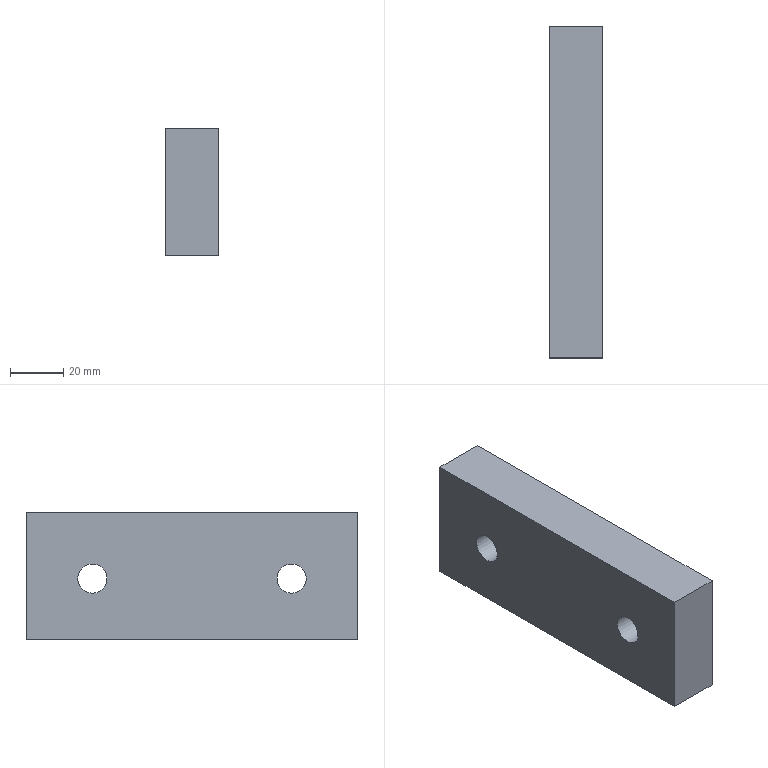Part | NX | features solid 2 | 1 solid | 12 faces | box 20 x 125 x 48 mm | volume 114744 mm3 | plane 8 | cylinder 4 | commonest cylinder face diameters 11 x2 17.5 x2
STEP:
#1=CARTESIAN_POINT('',(600.,560.,92.));
#2=VERTEX_POINT('',#1);
#3=CARTESIAN_POINT('',(580.,560.,92.));
#4=VERTEX_POINT('',#3);
#5=CARTESIAN_POINT('',(590.,560.,92.));
#6=DIRECTION('',(-1.,0.,0.));
#7=VECTOR('',#6,1000.);
#8=LINE('',#5,#7);
#9=EDGE_CURVE('',#2,#4,#8,.T.);
#10=ORIENTED_EDGE('',*,*,#9,.F.);
#11=CARTESIAN_POINT('',(600.,560.,140.));
#12=VERTEX_POINT('',#11);
#13=CARTESIAN_POINT('',(600.,560.,90.));
#14=DIRECTION('',(0.,0.,-1.));
#15=VECTOR('',#14,1000.);
#16=LINE('',#13,#15);
#17=EDGE_CURVE('',#12,#2,#16,.T.);
#18=ORIENTED_EDGE('',*,*,#17,.F.);
#19=CARTESIAN_POINT('',(580.,560.,140.));
#20=VERTEX_POINT('',#19);
#21=CARTESIAN_POINT('',(590.,560.,140.));
#22=DIRECTION('',(1.,0.,0.));
#23=VECTOR('',#22,1000.);
#24=LINE('',#21,#23);
#25=EDGE_CURVE('',#20,#12,#24,.T.);
#26=ORIENTED_EDGE('',*,*,#25,.F.);
#27=CARTESIAN_POINT('',(580.,560.,90.));
#28=DIRECTION('',(0.,0.,1.));
#29=VECTOR('',#28,1000.);
#30=LINE('',#27,#29);
#31=EDGE_CURVE('',#4,#20,#30,.T.);
#32=ORIENTED_EDGE('',*,*,#31,.F.);
#33=EDGE_LOOP('',(#10,#18,#26,#32));
#34=FACE_BOUND('',#33,.T.);
#35=CARTESIAN_POINT('',(590.,560.,90.));
#36=DIRECTION('',(0.,-1.,0.));
#37=DIRECTION('',(1.,0.,0.));
#38=AXIS2_PLACEMENT_3D('',#35,#36,#37);
#39=PLANE('',#38);
#40=ADVANCED_FACE('',(#34),#39,.T.);
#41=CARTESIAN_POINT('',(580.,685.,92.));
#42=VERTEX_POINT('',#41);
#43=CARTESIAN_POINT('',(580.,735.,92.));
#44=DIRECTION('',(0.,1.,0.));
#45=VECTOR('',#44,1000.);
#46=LINE('',#43,#45);
#47=EDGE_CURVE('',#4,#42,#46,.T.);
#48=ORIENTED_EDGE('',*,*,#47,.F.);
#49=ORIENTED_EDGE('',*,*,#31,.T.);
#50=CARTESIAN_POINT('',(580.,685.,140.));
#51=VERTEX_POINT('',#50);
#52=CARTESIAN_POINT('',(580.,735.,140.));
#53=DIRECTION('',(0.,-1.,0.));
#54=VECTOR('',#53,1000.);
#55=LINE('',#52,#54);
#56=EDGE_CURVE('',#51,#20,#55,.T.);
#57=ORIENTED_EDGE('',*,*,#56,.F.);
#58=CARTESIAN_POINT('',(580.,685.,90.));
#59=DIRECTION('',(0.,0.,-1.));
#60=VECTOR('',#59,1000.);
#61=LINE('',#58,#60);
#62=EDGE_CURVE('',#51,#42,#61,.T.);
#63=ORIENTED_EDGE('',*,*,#62,.T.);
#64=EDGE_LOOP('',(#48,#49,#57,#63));
#65=FACE_BOUND('',#64,.T.);
#66=CARTESIAN_POINT('',(580.,660.,120.5));
#67=VERTEX_POINT('',#66);
#68=CARTESIAN_POINT('',(580.,660.,115.));
#69=DIRECTION('',(-1.,0.,0.));
#70=DIRECTION('',(0.,0.,1.));
#71=AXIS2_PLACEMENT_3D('',#68,#69,#70);
#72=CIRCLE('',#71,5.5);
#73=EDGE_CURVE('',#67,#67,#72,.F.);
#74=ORIENTED_EDGE('',*,*,#73,.T.);
#75=EDGE_LOOP('',(#74));
#76=FACE_BOUND('',#75,.T.);
#77=CARTESIAN_POINT('',(580.,585.,120.5));
#78=VERTEX_POINT('',#77);
#79=CARTESIAN_POINT('',(580.,585.,115.));
#80=DIRECTION('',(-1.,0.,0.));
#81=DIRECTION('',(0.,0.,1.));
#82=AXIS2_PLACEMENT_3D('',#79,#80,#81);
#83=CIRCLE('',#82,5.5);
#84=EDGE_CURVE('',#78,#78,#83,.F.);
#85=ORIENTED_EDGE('',*,*,#84,.T.);
#86=EDGE_LOOP('',(#85));
#87=FACE_BOUND('',#86,.T.);
#88=CARTESIAN_POINT('',(580.,735.,90.));
#89=DIRECTION('',(-1.,0.,0.));
#90=DIRECTION('',(0.,-1.,0.));
#91=AXIS2_PLACEMENT_3D('',#88,#89,#90);
#92=PLANE('',#91);
#93=ADVANCED_FACE('',(#65,#76,#87),#92,.T.);
#94=ORIENTED_EDGE('',*,*,#56,.T.);
#95=ORIENTED_EDGE('',*,*,#25,.T.);
#96=CARTESIAN_POINT('',(600.,685.,140.));
#97=VERTEX_POINT('',#96);
#98=CARTESIAN_POINT('',(600.,735.,140.));
#99=DIRECTION('',(0.,-1.,0.));
#100=VECTOR('',#99,1000.);
#101=LINE('',#98,#100);
#102=EDGE_CURVE('',#97,#12,#101,.T.);
#103=ORIENTED_EDGE('',*,*,#102,.F.);
#104=CARTESIAN_POINT('',(590.,685.,140.));
#105=DIRECTION('',(-1.,0.,0.));
#106=VECTOR('',#105,1000.);
#107=LINE('',#104,#106);
#108=EDGE_CURVE('',#97,#51,#107,.T.);
#109=ORIENTED_EDGE('',*,*,#108,.T.);
#110=EDGE_LOOP('',(#94,#95,#103,#109));
#111=FACE_BOUND('',#110,.T.);
#112=CARTESIAN_POINT('',(590.,735.,140.));
#113=DIRECTION('',(0.,0.,1.));
#114=DIRECTION('',(0.,-1.,0.));
#115=AXIS2_PLACEMENT_3D('',#112,#113,#114);
#116=PLANE('',#115);
#117=ADVANCED_FACE('',(#111),#116,.T.);
#118=CARTESIAN_POINT('',(600.,685.,92.));
#119=VERTEX_POINT('',#118);
#120=CARTESIAN_POINT('',(590.,685.,92.));
#121=DIRECTION('',(1.,0.,0.));
#122=VECTOR('',#121,1000.);
#123=LINE('',#120,#122);
#124=EDGE_CURVE('',#42,#119,#123,.T.);
#125=ORIENTED_EDGE('',*,*,#124,.F.);
#126=ORIENTED_EDGE('',*,*,#62,.F.);
#127=ORIENTED_EDGE('',*,*,#108,.F.);
#128=CARTESIAN_POINT('',(600.,685.,90.));
#129=DIRECTION('',(0.,0.,1.));
#130=VECTOR('',#129,1000.);
#131=LINE('',#128,#130);
#132=EDGE_CURVE('',#119,#97,#131,.T.);
#133=ORIENTED_EDGE('',*,*,#132,.F.);
#134=EDGE_LOOP('',(#125,#126,#127,#133));
#135=FACE_BOUND('',#134,.T.);
#136=CARTESIAN_POINT('',(590.,685.,90.));
#137=DIRECTION('',(0.,1.,0.));
#138=DIRECTION('',(-1.,0.,0.));
#139=AXIS2_PLACEMENT_3D('',#136,#137,#138);
#140=PLANE('',#139);
#141=ADVANCED_FACE('',(#135),#140,.T.);
#142=CARTESIAN_POINT('',(600.,735.,92.));
#143=DIRECTION('',(0.,-1.,0.));
#144=VECTOR('',#143,1000.);
#145=LINE('',#142,#144);
#146=EDGE_CURVE('',#119,#2,#145,.T.);
#147=ORIENTED_EDGE('',*,*,#146,.F.);
#148=ORIENTED_EDGE('',*,*,#132,.T.);
#149=ORIENTED_EDGE('',*,*,#102,.T.);
#150=ORIENTED_EDGE('',*,*,#17,.T.);
#151=EDGE_LOOP('',(#147,#148,#149,#150));
#152=FACE_BOUND('',#151,.T.);
#153=CARTESIAN_POINT('',(600.,651.25,115.));
#154=VERTEX_POINT('',#153);
#155=CARTESIAN_POINT('',(600.,660.,115.));
#156=DIRECTION('',(-1.,0.,0.));
#157=DIRECTION('',(0.,-1.,0.));
#158=AXIS2_PLACEMENT_3D('',#155,#156,#157);
#159=CIRCLE('',#158,8.75);
#160=EDGE_CURVE('',#154,#154,#159,.T.);
#161=ORIENTED_EDGE('',*,*,#160,.T.);
#162=EDGE_LOOP('',(#161));
#163=FACE_BOUND('',#162,.T.);
#164=CARTESIAN_POINT('',(600.,576.25,115.));
#165=VERTEX_POINT('',#164);
#166=CARTESIAN_POINT('',(600.,585.,115.));
#167=DIRECTION('',(-1.,0.,0.));
#168=DIRECTION('',(0.,-1.,0.));
#169=AXIS2_PLACEMENT_3D('',#166,#167,#168);
#170=CIRCLE('',#169,8.75);
#171=EDGE_CURVE('',#165,#165,#170,.T.);
#172=ORIENTED_EDGE('',*,*,#171,.T.);
#173=EDGE_LOOP('',(#172));
#174=FACE_BOUND('',#173,.T.);
#175=CARTESIAN_POINT('',(600.,735.,90.));
#176=DIRECTION('',(1.,0.,0.));
#177=DIRECTION('',(0.,1.,0.));
#178=AXIS2_PLACEMENT_3D('',#175,#176,#177);
#179=PLANE('',#178);
#180=ADVANCED_FACE('',(#152,#163,#174),#179,.T.);
#181=CARTESIAN_POINT('',(595.,585.,120.5));
#182=VERTEX_POINT('',#181);
#183=CARTESIAN_POINT('',(595.,585.,115.));
#184=DIRECTION('',(-1.,0.,0.));
#185=DIRECTION('',(0.,0.,1.));
#186=AXIS2_PLACEMENT_3D('',#183,#184,#185);
#187=CIRCLE('',#186,5.5);
#188=EDGE_CURVE('',#182,#182,#187,.F.);
#189=ORIENTED_EDGE('',*,*,#188,.T.);
#190=EDGE_LOOP('',(#189));
#191=FACE_BOUND('',#190,.T.);
#192=ORIENTED_EDGE('',*,*,#84,.F.);
#193=EDGE_LOOP('',(#192));
#194=FACE_BOUND('',#193,.T.);
#195=CARTESIAN_POINT('',(580.,585.,115.));
#196=DIRECTION('',(1.,0.,0.));
#197=DIRECTION('',(0.,1.,0.));
#198=AXIS2_PLACEMENT_3D('',#195,#196,#197);
#199=CYLINDRICAL_SURFACE('',#198,5.5);
#200=ADVANCED_FACE('',(#191,#194),#199,.F.);
#201=CARTESIAN_POINT('',(595.,585.,123.75));
#202=VERTEX_POINT('',#201);
#203=CARTESIAN_POINT('',(595.,585.,115.));
#204=DIRECTION('',(-1.,0.,0.));
#205=DIRECTION('',(0.,0.,1.));
#206=AXIS2_PLACEMENT_3D('',#203,#204,#205);
#207=CIRCLE('',#206,8.75);
#208=EDGE_CURVE('',#202,#202,#207,.F.);
#209=ORIENTED_EDGE('',*,*,#208,.T.);
#210=EDGE_LOOP('',(#209));
#211=FACE_BOUND('',#210,.T.);
#212=ORIENTED_EDGE('',*,*,#188,.F.);
#213=EDGE_LOOP('',(#212));
#214=FACE_BOUND('',#213,.T.);
#215=CARTESIAN_POINT('',(595.,585.,115.));
#216=DIRECTION('',(-1.,0.,0.));
#217=DIRECTION('',(0.,-1.,0.));
#218=AXIS2_PLACEMENT_3D('',#215,#216,#217);
#219=PLANE('',#218);
#220=ADVANCED_FACE('',(#211,#214),#219,.F.);
#221=ORIENTED_EDGE('',*,*,#171,.F.);
#222=EDGE_LOOP('',(#221));
#223=FACE_BOUND('',#222,.T.);
#224=ORIENTED_EDGE('',*,*,#208,.F.);
#225=EDGE_LOOP('',(#224));
#226=FACE_BOUND('',#225,.T.);
#227=CARTESIAN_POINT('',(585.,585.,115.));
#228=DIRECTION('',(1.,0.,0.));
#229=DIRECTION('',(0.,1.,0.));
#230=AXIS2_PLACEMENT_3D('',#227,#228,#229);
#231=CYLINDRICAL_SURFACE('',#230,8.75);
#232=ADVANCED_FACE('',(#223,#226),#231,.F.);
#233=CARTESIAN_POINT('',(595.,660.,120.5));
#234=VERTEX_POINT('',#233);
#235=CARTESIAN_POINT('',(595.,660.,115.));
#236=DIRECTION('',(-1.,0.,0.));
#237=DIRECTION('',(0.,0.,1.));
#238=AXIS2_PLACEMENT_3D('',#235,#236,#237);
#239=CIRCLE('',#238,5.5);
#240=EDGE_CURVE('',#234,#234,#239,.F.);
#241=ORIENTED_EDGE('',*,*,#240,.T.);
#242=EDGE_LOOP('',(#241));
#243=FACE_BOUND('',#242,.T.);
#244=ORIENTED_EDGE('',*,*,#73,.F.);
#245=EDGE_LOOP('',(#244));
#246=FACE_BOUND('',#245,.T.);
#247=CARTESIAN_POINT('',(580.,660.,115.));
#248=DIRECTION('',(1.,0.,0.));
#249=DIRECTION('',(0.,1.,0.));
#250=AXIS2_PLACEMENT_3D('',#247,#248,#249);
#251=CYLINDRICAL_SURFACE('',#250,5.5);
#252=ADVANCED_FACE('',(#243,#246),#251,.F.);
#253=CARTESIAN_POINT('',(595.,660.,123.75));
#254=VERTEX_POINT('',#253);
#255=CARTESIAN_POINT('',(595.,660.,115.));
#256=DIRECTION('',(-1.,0.,0.));
#257=DIRECTION('',(0.,0.,1.));
#258=AXIS2_PLACEMENT_3D('',#255,#256,#257);
#259=CIRCLE('',#258,8.75);
#260=EDGE_CURVE('',#254,#254,#259,.F.);
#261=ORIENTED_EDGE('',*,*,#260,.T.);
#262=EDGE_LOOP('',(#261));
#263=FACE_BOUND('',#262,.T.);
#264=ORIENTED_EDGE('',*,*,#240,.F.);
#265=EDGE_LOOP('',(#264));
#266=FACE_BOUND('',#265,.T.);
#267=CARTESIAN_POINT('',(595.,660.,115.));
#268=DIRECTION('',(-1.,0.,0.));
#269=DIRECTION('',(0.,-1.,0.));
#270=AXIS2_PLACEMENT_3D('',#267,#268,#269);
#271=PLANE('',#270);
#272=ADVANCED_FACE('',(#263,#266),#271,.F.);
#273=ORIENTED_EDGE('',*,*,#160,.F.);
#274=EDGE_LOOP('',(#273));
#275=FACE_BOUND('',#274,.T.);
#276=ORIENTED_EDGE('',*,*,#260,.F.);
#277=EDGE_LOOP('',(#276));
#278=FACE_BOUND('',#277,.T.);
#279=CARTESIAN_POINT('',(585.,660.,115.));
#280=DIRECTION('',(1.,0.,0.));
#281=DIRECTION('',(0.,1.,0.));
#282=AXIS2_PLACEMENT_3D('',#279,#280,#281);
#283=CYLINDRICAL_SURFACE('',#282,8.75);
#284=ADVANCED_FACE('',(#275,#278),#283,.F.);
#285=ORIENTED_EDGE('',*,*,#9,.T.);
#286=ORIENTED_EDGE('',*,*,#47,.T.);
#287=ORIENTED_EDGE('',*,*,#124,.T.);
#288=ORIENTED_EDGE('',*,*,#146,.T.);
#289=EDGE_LOOP('',(#285,#286,#287,#288));
#290=FACE_BOUND('',#289,.T.);
#291=CARTESIAN_POINT('',(580.,485.,92.));
#292=DIRECTION('',(0.,0.,1.));
#293=DIRECTION('',(1.,0.,0.));
#294=AXIS2_PLACEMENT_3D('',#291,#292,#293);
#295=PLANE('',#294);
#296=ADVANCED_FACE('',(#290),#295,.F.);
#297=CLOSED_SHELL('',(#40,#93,#117,#141,#180,#200,#220,#232,#252,#272,#284,#296));
#298=MANIFOLD_SOLID_BREP('',#297);
#299=(LENGTH_UNIT()NAMED_UNIT(*)SI_UNIT(.MILLI.,.METRE.));
#300=UNCERTAINTY_MEASURE_WITH_UNIT(LENGTH_MEASURE(0.00001),#299,'','');
#301=(NAMED_UNIT(*)PLANE_ANGLE_UNIT()SI_UNIT($,.RADIAN.));
#302=(NAMED_UNIT(*)SI_UNIT($,.STERADIAN.)SOLID_ANGLE_UNIT());
#303=(GEOMETRIC_REPRESENTATION_CONTEXT(3)GLOBAL_UNCERTAINTY_ASSIGNED_CONTEXT((#300))GLOBAL_UNIT_ASSIGNED_CONTEXT((#299,#301,#302))REPRESENTATION_CONTEXT('',''));
#304=ADVANCED_BREP_SHAPE_REPRESENTATION('',(#298),#303);